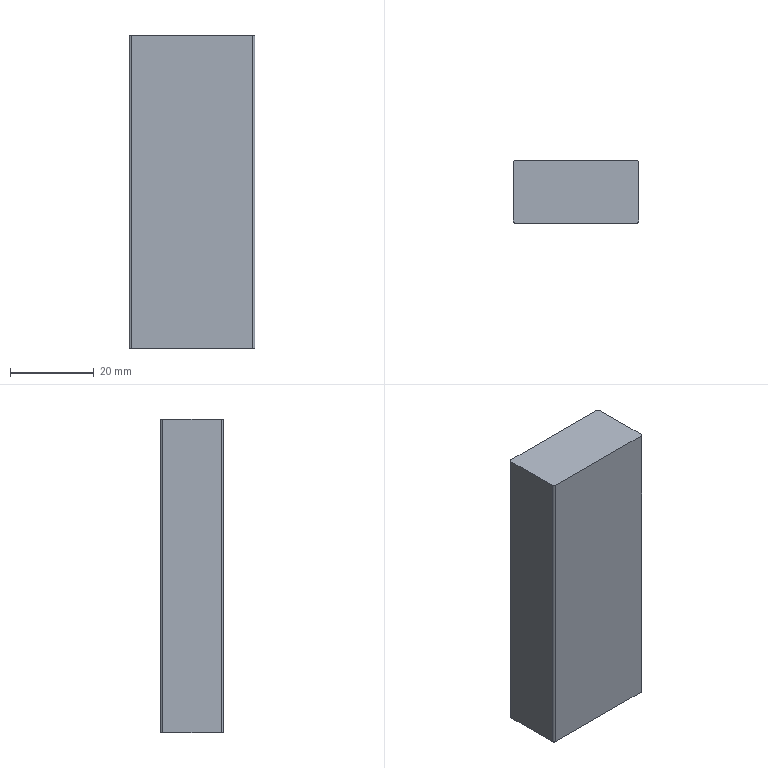Part | STEP file | 1 solid | 88 faces | box 30 x 15 x 75 mm | volume 32980 mm3 | plane 57 | other 24 | cylinder 5 | cone 2 | commonest cylinder face diameters 1 x4 5 x1